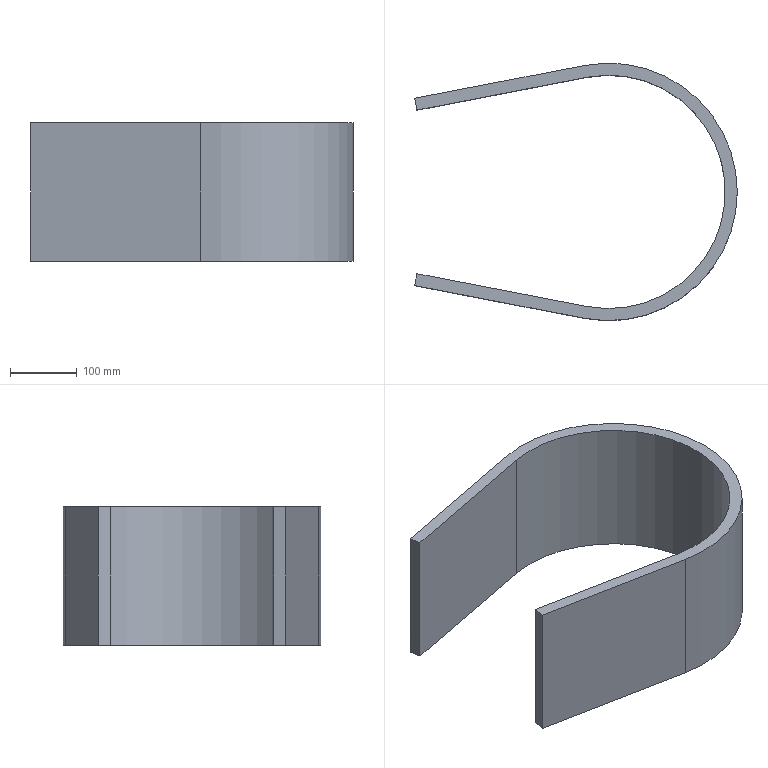Part | SolidWorks | features Extrusion 1 | 1 solid | 10 faces | box 482.5 x 385 x 207.5 mm | volume 4343346 mm3 | plane 8 | cylinder 2 | commonest cylinder face diameters 349 x1 385 x1
STEP:
#1=CARTESIAN_POINT('',(-286.583,-122.327,0.));
#2=VERTEX_POINT('',#1);
#3=CARTESIAN_POINT('',(-290.,-140.,0.));
#4=VERTEX_POINT('',#3);
#5=CARTESIAN_POINT('',(-286.583,-122.327,0.));
#6=DIRECTION('',(-0.1898,-0.9818,0.));
#7=VECTOR('',#6,1000.);
#8=LINE('',#5,#7);
#9=EDGE_CURVE('',#2,#4,#8,.T.);
#10=ORIENTED_EDGE('',*,*,#9,.T.);
#11=CARTESIAN_POINT('',(-290.,-140.,207.5));
#12=VERTEX_POINT('',#11);
#13=CARTESIAN_POINT('',(-290.,-140.,207.5));
#14=DIRECTION('',(0.,0.,-1.));
#15=VECTOR('',#14,1000.);
#16=LINE('',#13,#15);
#17=EDGE_CURVE('',#12,#4,#16,.T.);
#18=ORIENTED_EDGE('',*,*,#17,.F.);
#19=CARTESIAN_POINT('',(-286.583,-122.327,207.5));
#20=VERTEX_POINT('',#19);
#21=CARTESIAN_POINT('',(-286.583,-122.327,207.5));
#22=DIRECTION('',(-0.1898,-0.9818,0.));
#23=VECTOR('',#22,1000.);
#24=LINE('',#21,#23);
#25=EDGE_CURVE('',#20,#12,#24,.T.);
#26=ORIENTED_EDGE('',*,*,#25,.F.);
#27=CARTESIAN_POINT('',(-286.583,-122.327,207.5));
#28=DIRECTION('',(0.,0.,-1.));
#29=VECTOR('',#28,1000.);
#30=LINE('',#27,#29);
#31=EDGE_CURVE('',#20,#2,#30,.T.);
#32=ORIENTED_EDGE('',*,*,#31,.T.);
#33=EDGE_LOOP('',(#10,#18,#26,#32));
#34=FACE_OUTER_BOUND('',#33,.T.);
#35=CARTESIAN_POINT('',(-286.583,-122.327,207.5));
#36=DIRECTION('',(0.9818,-0.1898,0.));
#37=DIRECTION('',(0.1898,0.9818,0.));
#38=AXIS2_PLACEMENT_3D('',#35,#36,#37);
#39=PLANE('',#38);
#40=ADVANCED_FACE('',(#34),#39,.F.);
#41=CARTESIAN_POINT('',(-36.539,-189.,0.));
#42=VERTEX_POINT('',#41);
#43=CARTESIAN_POINT('',(-290.,-140.,0.));
#44=DIRECTION('',(0.9818,-0.1898,0.));
#45=VECTOR('',#44,1000.);
#46=LINE('',#43,#45);
#47=EDGE_CURVE('',#4,#42,#46,.T.);
#48=ORIENTED_EDGE('',*,*,#47,.T.);
#49=CARTESIAN_POINT('',(-36.539,-189.,207.5));
#50=VERTEX_POINT('',#49);
#51=CARTESIAN_POINT('',(-36.539,-189.,207.5));
#52=DIRECTION('',(0.,0.,-1.));
#53=VECTOR('',#52,1000.);
#54=LINE('',#51,#53);
#55=EDGE_CURVE('',#50,#42,#54,.T.);
#56=ORIENTED_EDGE('',*,*,#55,.F.);
#57=CARTESIAN_POINT('',(-290.,-140.,207.5));
#58=DIRECTION('',(0.9818,-0.1898,0.));
#59=VECTOR('',#58,1000.);
#60=LINE('',#57,#59);
#61=EDGE_CURVE('',#12,#50,#60,.T.);
#62=ORIENTED_EDGE('',*,*,#61,.F.);
#63=ORIENTED_EDGE('',*,*,#17,.T.);
#64=EDGE_LOOP('',(#48,#56,#62,#63));
#65=FACE_OUTER_BOUND('',#64,.T.);
#66=CARTESIAN_POINT('',(-290.,-140.,207.5));
#67=DIRECTION('',(0.1898,0.9818,0.));
#68=DIRECTION('',(-0.9818,0.1898,0.));
#69=AXIS2_PLACEMENT_3D('',#66,#67,#68);
#70=PLANE('',#69);
#71=ADVANCED_FACE('',(#65),#70,.F.);
#72=CARTESIAN_POINT('',(-36.539,189.,0.));
#73=VERTEX_POINT('',#72);
#74=CARTESIAN_POINT('',(0.,0.,0.));
#75=DIRECTION('',(0.,0.,1.));
#76=DIRECTION('',(1.,0.,0.));
#77=AXIS2_PLACEMENT_3D('',#74,#75,#76);
#78=CIRCLE('',#77,192.5);
#79=EDGE_CURVE('',#42,#73,#78,.T.);
#80=ORIENTED_EDGE('',*,*,#79,.T.);
#81=CARTESIAN_POINT('',(-36.539,189.,207.5));
#82=VERTEX_POINT('',#81);
#83=CARTESIAN_POINT('',(-36.539,189.,207.5));
#84=DIRECTION('',(0.,0.,-1.));
#85=VECTOR('',#84,1000.);
#86=LINE('',#83,#85);
#87=EDGE_CURVE('',#82,#73,#86,.T.);
#88=ORIENTED_EDGE('',*,*,#87,.F.);
#89=CARTESIAN_POINT('',(0.,0.,207.5));
#90=DIRECTION('',(0.,0.,1.));
#91=DIRECTION('',(1.,0.,0.));
#92=AXIS2_PLACEMENT_3D('',#89,#90,#91);
#93=CIRCLE('',#92,192.5);
#94=EDGE_CURVE('',#50,#82,#93,.T.);
#95=ORIENTED_EDGE('',*,*,#94,.F.);
#96=ORIENTED_EDGE('',*,*,#55,.T.);
#97=EDGE_LOOP('',(#80,#88,#95,#96));
#98=FACE_OUTER_BOUND('',#97,.T.);
#99=CARTESIAN_POINT('',(0.,0.,207.5));
#100=DIRECTION('',(0.,0.,-1.));
#101=DIRECTION('',(-1.,0.,0.));
#102=AXIS2_PLACEMENT_3D('',#99,#100,#101);
#103=CYLINDRICAL_SURFACE('',#102,192.5);
#104=ADVANCED_FACE('',(#98),#103,.T.);
#105=CARTESIAN_POINT('',(-290.,140.,0.));
#106=VERTEX_POINT('',#105);
#107=CARTESIAN_POINT('',(-290.,140.,0.));
#108=DIRECTION('',(-0.9818,-0.1898,0.));
#109=VECTOR('',#108,1000.);
#110=LINE('',#107,#109);
#111=EDGE_CURVE('',#73,#106,#110,.T.);
#112=ORIENTED_EDGE('',*,*,#111,.T.);
#113=CARTESIAN_POINT('',(-290.,140.,207.5));
#114=VERTEX_POINT('',#113);
#115=CARTESIAN_POINT('',(-290.,140.,207.5));
#116=DIRECTION('',(0.,0.,-1.));
#117=VECTOR('',#116,1000.);
#118=LINE('',#115,#117);
#119=EDGE_CURVE('',#114,#106,#118,.T.);
#120=ORIENTED_EDGE('',*,*,#119,.F.);
#121=CARTESIAN_POINT('',(-290.,140.,207.5));
#122=DIRECTION('',(-0.9818,-0.1898,0.));
#123=VECTOR('',#122,1000.);
#124=LINE('',#121,#123);
#125=EDGE_CURVE('',#82,#114,#124,.T.);
#126=ORIENTED_EDGE('',*,*,#125,.F.);
#127=ORIENTED_EDGE('',*,*,#87,.T.);
#128=EDGE_LOOP('',(#112,#120,#126,#127));
#129=FACE_OUTER_BOUND('',#128,.T.);
#130=CARTESIAN_POINT('',(-290.,140.,207.5));
#131=DIRECTION('',(0.1898,-0.9818,0.));
#132=DIRECTION('',(0.9818,0.1898,0.));
#133=AXIS2_PLACEMENT_3D('',#130,#131,#132);
#134=PLANE('',#133);
#135=ADVANCED_FACE('',(#129),#134,.F.);
#136=CARTESIAN_POINT('',(-286.583,122.327,0.));
#137=VERTEX_POINT('',#136);
#138=CARTESIAN_POINT('',(-290.,140.,0.));
#139=DIRECTION('',(0.1898,-0.9818,0.));
#140=VECTOR('',#139,1000.);
#141=LINE('',#138,#140);
#142=EDGE_CURVE('',#106,#137,#141,.T.);
#143=ORIENTED_EDGE('',*,*,#142,.T.);
#144=CARTESIAN_POINT('',(-286.583,122.327,207.5));
#145=VERTEX_POINT('',#144);
#146=CARTESIAN_POINT('',(-286.583,122.327,207.5));
#147=DIRECTION('',(0.,0.,-1.));
#148=VECTOR('',#147,1000.);
#149=LINE('',#146,#148);
#150=EDGE_CURVE('',#145,#137,#149,.T.);
#151=ORIENTED_EDGE('',*,*,#150,.F.);
#152=CARTESIAN_POINT('',(-290.,140.,207.5));
#153=DIRECTION('',(0.1898,-0.9818,0.));
#154=VECTOR('',#153,1000.);
#155=LINE('',#152,#154);
#156=EDGE_CURVE('',#114,#145,#155,.T.);
#157=ORIENTED_EDGE('',*,*,#156,.F.);
#158=ORIENTED_EDGE('',*,*,#119,.T.);
#159=EDGE_LOOP('',(#143,#151,#157,#158));
#160=FACE_OUTER_BOUND('',#159,.T.);
#161=CARTESIAN_POINT('',(-290.,140.,207.5));
#162=DIRECTION('',(0.9818,0.1898,0.));
#163=DIRECTION('',(-0.1898,0.9818,0.));
#164=AXIS2_PLACEMENT_3D('',#161,#162,#163);
#165=PLANE('',#164);
#166=ADVANCED_FACE('',(#160),#165,.F.);
#167=CARTESIAN_POINT('',(-33.122,171.328,0.));
#168=VERTEX_POINT('',#167);
#169=CARTESIAN_POINT('',(-286.583,122.327,0.));
#170=DIRECTION('',(0.9818,0.1898,0.));
#171=VECTOR('',#170,1000.);
#172=LINE('',#169,#171);
#173=EDGE_CURVE('',#137,#168,#172,.T.);
#174=ORIENTED_EDGE('',*,*,#173,.T.);
#175=CARTESIAN_POINT('',(-33.122,171.328,207.5));
#176=VERTEX_POINT('',#175);
#177=CARTESIAN_POINT('',(-33.122,171.328,207.5));
#178=DIRECTION('',(0.,0.,-1.));
#179=VECTOR('',#178,1000.);
#180=LINE('',#177,#179);
#181=EDGE_CURVE('',#176,#168,#180,.T.);
#182=ORIENTED_EDGE('',*,*,#181,.F.);
#183=CARTESIAN_POINT('',(-286.583,122.327,207.5));
#184=DIRECTION('',(0.9818,0.1898,0.));
#185=VECTOR('',#184,1000.);
#186=LINE('',#183,#185);
#187=EDGE_CURVE('',#145,#176,#186,.T.);
#188=ORIENTED_EDGE('',*,*,#187,.F.);
#189=ORIENTED_EDGE('',*,*,#150,.T.);
#190=EDGE_LOOP('',(#174,#182,#188,#189));
#191=FACE_OUTER_BOUND('',#190,.T.);
#192=CARTESIAN_POINT('',(-286.583,122.327,207.5));
#193=DIRECTION('',(-0.1898,0.9818,0.));
#194=DIRECTION('',(-0.9818,-0.1898,0.));
#195=AXIS2_PLACEMENT_3D('',#192,#193,#194);
#196=PLANE('',#195);
#197=ADVANCED_FACE('',(#191),#196,.F.);
#198=CARTESIAN_POINT('',(-33.122,-171.328,0.));
#199=VERTEX_POINT('',#198);
#200=CARTESIAN_POINT('',(0.,0.,0.));
#201=DIRECTION('',(0.,0.,-1.));
#202=DIRECTION('',(1.,0.,0.));
#203=AXIS2_PLACEMENT_3D('',#200,#201,#202);
#204=CIRCLE('',#203,174.5);
#205=EDGE_CURVE('',#168,#199,#204,.T.);
#206=ORIENTED_EDGE('',*,*,#205,.T.);
#207=CARTESIAN_POINT('',(-33.122,-171.328,207.5));
#208=VERTEX_POINT('',#207);
#209=CARTESIAN_POINT('',(-33.122,-171.328,207.5));
#210=DIRECTION('',(0.,0.,-1.));
#211=VECTOR('',#210,1000.);
#212=LINE('',#209,#211);
#213=EDGE_CURVE('',#208,#199,#212,.T.);
#214=ORIENTED_EDGE('',*,*,#213,.F.);
#215=CARTESIAN_POINT('',(0.,0.,207.5));
#216=DIRECTION('',(0.,0.,-1.));
#217=DIRECTION('',(1.,0.,0.));
#218=AXIS2_PLACEMENT_3D('',#215,#216,#217);
#219=CIRCLE('',#218,174.5);
#220=EDGE_CURVE('',#176,#208,#219,.T.);
#221=ORIENTED_EDGE('',*,*,#220,.F.);
#222=ORIENTED_EDGE('',*,*,#181,.T.);
#223=EDGE_LOOP('',(#206,#214,#221,#222));
#224=FACE_OUTER_BOUND('',#223,.T.);
#225=CARTESIAN_POINT('',(0.,0.,207.5));
#226=DIRECTION('',(0.,0.,-1.));
#227=DIRECTION('',(-1.,0.,0.));
#228=AXIS2_PLACEMENT_3D('',#225,#226,#227);
#229=CYLINDRICAL_SURFACE('',#228,174.5);
#230=ADVANCED_FACE('',(#224),#229,.F.);
#231=CARTESIAN_POINT('',(-286.583,-122.327,0.));
#232=DIRECTION('',(-0.9818,0.1898,0.));
#233=VECTOR('',#232,1000.);
#234=LINE('',#231,#233);
#235=EDGE_CURVE('',#199,#2,#234,.T.);
#236=ORIENTED_EDGE('',*,*,#235,.T.);
#237=ORIENTED_EDGE('',*,*,#31,.F.);
#238=CARTESIAN_POINT('',(-286.583,-122.327,207.5));
#239=DIRECTION('',(-0.9818,0.1898,0.));
#240=VECTOR('',#239,1000.);
#241=LINE('',#238,#240);
#242=EDGE_CURVE('',#208,#20,#241,.T.);
#243=ORIENTED_EDGE('',*,*,#242,.F.);
#244=ORIENTED_EDGE('',*,*,#213,.T.);
#245=EDGE_LOOP('',(#236,#237,#243,#244));
#246=FACE_OUTER_BOUND('',#245,.T.);
#247=CARTESIAN_POINT('',(-286.583,-122.327,207.5));
#248=DIRECTION('',(-0.1898,-0.9818,0.));
#249=DIRECTION('',(0.9818,-0.1898,0.));
#250=AXIS2_PLACEMENT_3D('',#247,#248,#249);
#251=PLANE('',#250);
#252=ADVANCED_FACE('',(#246),#251,.F.);
#253=ORIENTED_EDGE('',*,*,#25,.T.);
#254=ORIENTED_EDGE('',*,*,#61,.T.);
#255=ORIENTED_EDGE('',*,*,#94,.T.);
#256=ORIENTED_EDGE('',*,*,#125,.T.);
#257=ORIENTED_EDGE('',*,*,#156,.T.);
#258=ORIENTED_EDGE('',*,*,#187,.T.);
#259=ORIENTED_EDGE('',*,*,#220,.T.);
#260=ORIENTED_EDGE('',*,*,#242,.T.);
#261=EDGE_LOOP('',(#253,#254,#255,#256,#257,#258,#259,#260));
#262=FACE_OUTER_BOUND('',#261,.T.);
#263=CARTESIAN_POINT('',(0.,0.,207.5));
#264=DIRECTION('',(0.,0.,1.));
#265=DIRECTION('',(1.,0.,0.));
#266=AXIS2_PLACEMENT_3D('',#263,#264,#265);
#267=PLANE('',#266);
#268=ADVANCED_FACE('',(#262),#267,.T.);
#269=ORIENTED_EDGE('',*,*,#9,.F.);
#270=ORIENTED_EDGE('',*,*,#235,.F.);
#271=ORIENTED_EDGE('',*,*,#205,.F.);
#272=ORIENTED_EDGE('',*,*,#173,.F.);
#273=ORIENTED_EDGE('',*,*,#142,.F.);
#274=ORIENTED_EDGE('',*,*,#111,.F.);
#275=ORIENTED_EDGE('',*,*,#79,.F.);
#276=ORIENTED_EDGE('',*,*,#47,.F.);
#277=EDGE_LOOP('',(#269,#270,#271,#272,#273,#274,#275,#276));
#278=FACE_OUTER_BOUND('',#277,.T.);
#279=CARTESIAN_POINT('',(0.,0.,0.));
#280=DIRECTION('',(0.,0.,1.));
#281=DIRECTION('',(1.,0.,0.));
#282=AXIS2_PLACEMENT_3D('',#279,#280,#281);
#283=PLANE('',#282);
#284=ADVANCED_FACE('',(#278),#283,.F.);
#285=CLOSED_SHELL('',(#40,#71,#104,#135,#166,#197,#230,#252,#268,#284));
#286=MANIFOLD_SOLID_BREP('',#285);
#287=CARTESIAN_POINT('',(0.,0.,0.));
#288=DIRECTION('',(0.,0.,1.));
#289=DIRECTION('',(1.,0.,0.));
#290=AXIS2_PLACEMENT_3D('',#287,#288,#289);
#291=(LENGTH_UNIT()NAMED_UNIT(*)SI_UNIT(.MILLI.,.METRE.));
#292=UNCERTAINTY_MEASURE_WITH_UNIT(LENGTH_MEASURE(0.00001),#291,'','');
#293=(NAMED_UNIT(*)PLANE_ANGLE_UNIT()SI_UNIT($,.RADIAN.));
#294=(NAMED_UNIT(*)SI_UNIT($,.STERADIAN.)SOLID_ANGLE_UNIT());
#295=(GEOMETRIC_REPRESENTATION_CONTEXT(3)GLOBAL_UNCERTAINTY_ASSIGNED_CONTEXT((#292))GLOBAL_UNIT_ASSIGNED_CONTEXT((#291,#293,#294))REPRESENTATION_CONTEXT('',''));
#296=ADVANCED_BREP_SHAPE_REPRESENTATION('',(#286,#290),#295);